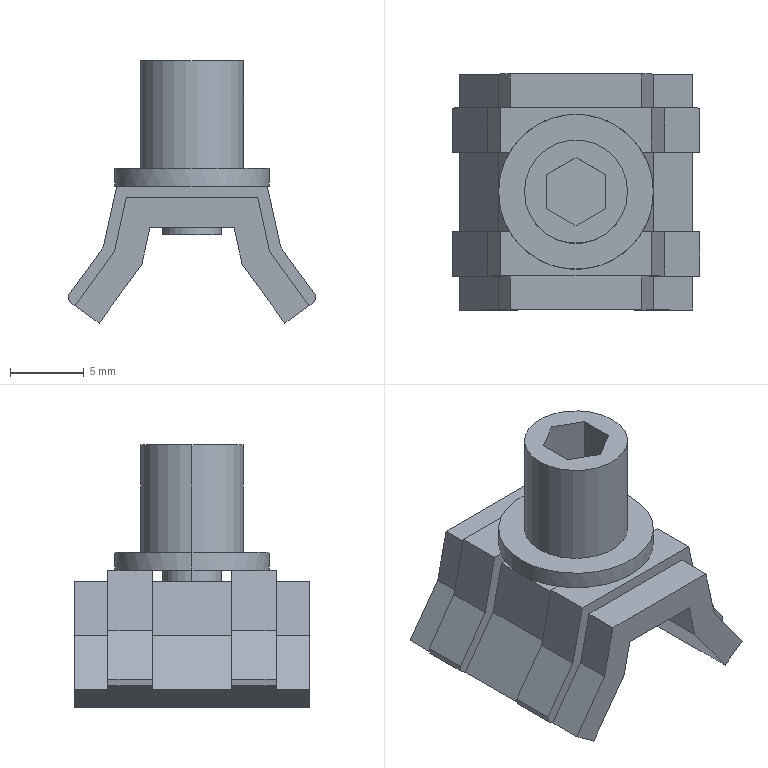Part | STEP file | _Y300T-A_FRONT | 1 solid | 61 faces | box 16.782 x 16 x 17.8 mm | volume 1225 mm3 | plane 53 | cylinder 8 | commonest cylinder face diameters 4 x4 7 x2 10.5 x2